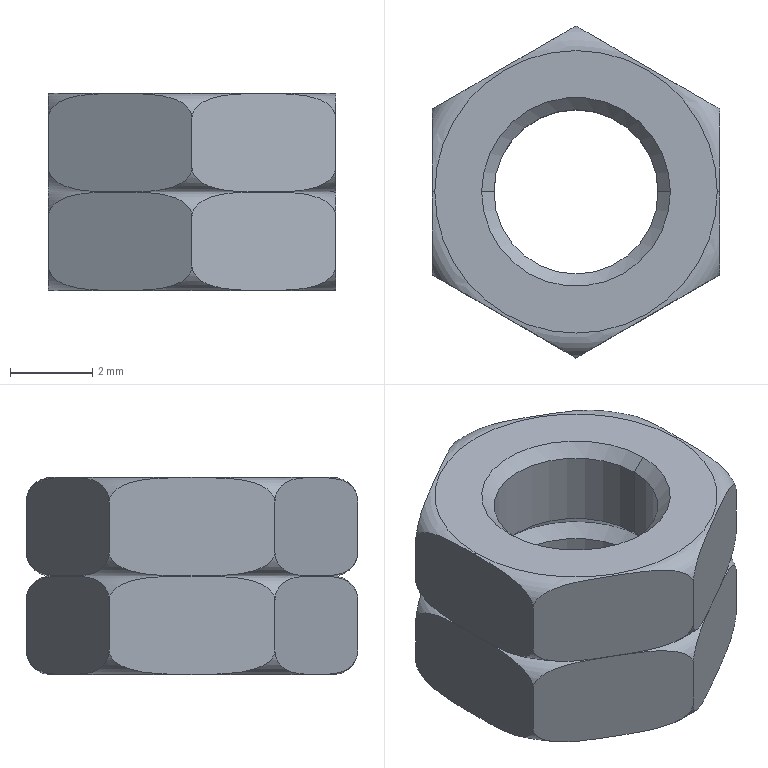Part | NX | 1 solid | 34 faces | box 7 x 8.083 x 4.8 mm | volume 140.02 mm3 | plane 14 | cone 8 | torus 8 | cylinder 4 | commonest cylinder face diameters 4 x4